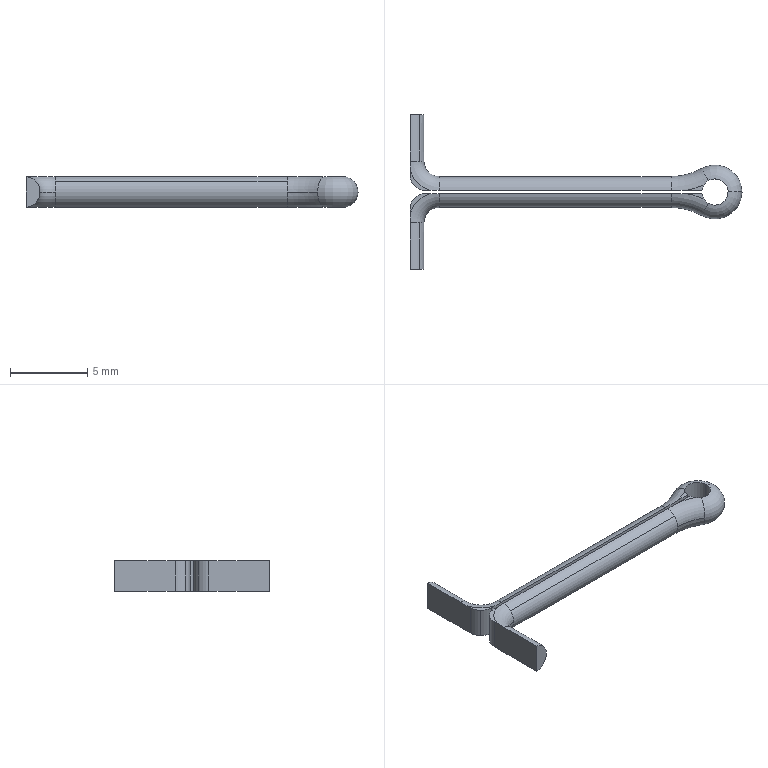Part | SolidWorks | features BaseBody 1 | 1 solid | 38 faces | box 21.489 x 10 x 2 mm | volume 72.863 mm3 | cylinder 14 | plane 14 | torus 10 | commonest cylinder face diameters 2 x12 1.7 x2
STEP:
#1=CARTESIAN_POINT('',(-17.839,-0.1,0.005013));
#2=VERTEX_POINT('',#1);
#3=CARTESIAN_POINT('',(-17.839,-1.,1.));
#4=VERTEX_POINT('',#3);
#5=CARTESIAN_POINT('',(-17.839,0.,1.));
#6=DIRECTION('',(-1.,0.,0.));
#7=DIRECTION('',(0.,0.,-1.));
#8=AXIS2_PLACEMENT_3D('',#5,#6,#7);
#9=CIRCLE('',#8,1.);
#10=EDGE_CURVE('',#2,#4,#9,.T.);
#11=ORIENTED_EDGE('',*,*,#10,.T.);
#12=CARTESIAN_POINT('',(-18.839,-2.,1.));
#13=VERTEX_POINT('',#12);
#14=CARTESIAN_POINT('',(-17.839,-2.,1.));
#15=DIRECTION('',(0.,0.,1.));
#16=DIRECTION('',(1.,0.,0.));
#17=AXIS2_PLACEMENT_3D('',#14,#15,#16);
#18=CIRCLE('',#17,1.);
#19=EDGE_CURVE('',#4,#13,#18,.T.);
#20=ORIENTED_EDGE('',*,*,#19,.T.);
#21=CARTESIAN_POINT('',(-19.739,-2.,0.005013));
#22=VERTEX_POINT('',#21);
#23=CARTESIAN_POINT('',(-19.839,-2.,1.));
#24=DIRECTION('',(0.,1.,0.));
#25=DIRECTION('',(1.,0.,0.));
#26=AXIS2_PLACEMENT_3D('',#23,#24,#25);
#27=CIRCLE('',#26,1.);
#28=EDGE_CURVE('',#13,#22,#27,.T.);
#29=ORIENTED_EDGE('',*,*,#28,.T.);
#30=CARTESIAN_POINT('',(-19.739,-1.376,0.));
#31=VERTEX_POINT('',#30);
#32=CARTESIAN_POINT('',(-19.739,-2.,0.005013));
#33=CARTESIAN_POINT('',(-19.739,-1.792,0.005013));
#34=CARTESIAN_POINT('',(-19.739,-1.584,0.));
#35=CARTESIAN_POINT('',(-19.739,-1.376,0.));
#36=B_SPLINE_CURVE_WITH_KNOTS('',3,(#32,#33,#34,#35),.UNSPECIFIED.,.F.,.F.,(4,4),(0.,0.0006245),.UNSPECIFIED.);
#37=EDGE_CURVE('',#22,#31,#36,.T.);
#38=ORIENTED_EDGE('',*,*,#37,.T.);
#39=CARTESIAN_POINT('',(-18.464,-0.1,0.));
#40=VERTEX_POINT('',#39);
#41=CARTESIAN_POINT('',(-17.839,-2.,0.));
#42=DIRECTION('',(0.,0.,-1.));
#43=DIRECTION('',(-0.7071,0.7071,0.));
#44=AXIS2_PLACEMENT_3D('',#41,#42,#43);
#45=CIRCLE('',#44,2.);
#46=EDGE_CURVE('',#31,#40,#45,.T.);
#47=ORIENTED_EDGE('',*,*,#46,.T.);
#48=CARTESIAN_POINT('',(-18.464,-0.1,0.));
#49=CARTESIAN_POINT('',(-18.256,-0.1,0.));
#50=CARTESIAN_POINT('',(-18.048,-0.1,0.005013));
#51=CARTESIAN_POINT('',(-17.839,-0.1,0.005013));
#52=B_SPLINE_CURVE_WITH_KNOTS('',3,(#48,#49,#50,#51),.UNSPECIFIED.,.F.,.F.,(4,4),(0.,0.0006245),.UNSPECIFIED.);
#53=EDGE_CURVE('',#40,#2,#52,.T.);
#54=ORIENTED_EDGE('',*,*,#53,.T.);
#55=EDGE_LOOP('',(#11,#20,#29,#38,#47,#54));
#56=FACE_OUTER_BOUND('',#55,.T.);
#57=CARTESIAN_POINT('',(-17.839,-2.,1.));
#58=DIRECTION('',(0.,0.,1.));
#59=DIRECTION('',(1.,0.,0.));
#60=AXIS2_PLACEMENT_3D('',#57,#58,#59);
#61=TOROIDAL_SURFACE('',#60,2.,1.);
#62=ADVANCED_FACE('',(#56),#61,.T.);
#63=CARTESIAN_POINT('',(-2.839,-0.7071,1.707));
#64=VERTEX_POINT('',#63);
#65=CARTESIAN_POINT('',(-2.839,-1.,1.));
#66=VERTEX_POINT('',#65);
#67=CARTESIAN_POINT('',(-2.839,0.,1.));
#68=DIRECTION('',(1.,0.,0.));
#69=DIRECTION('',(0.,-1.,0.));
#70=AXIS2_PLACEMENT_3D('',#67,#68,#69);
#71=CIRCLE('',#70,1.);
#72=EDGE_CURVE('',#64,#66,#71,.T.);
#73=ORIENTED_EDGE('',*,*,#72,.T.);
#74=CARTESIAN_POINT('',(-0.8642,-1.522,1.));
#75=VERTEX_POINT('',#74);
#76=CARTESIAN_POINT('',(-2.839,-5.,1.));
#77=DIRECTION('',(0.,0.,-1.));
#78=DIRECTION('',(-1.,0.,0.));
#79=AXIS2_PLACEMENT_3D('',#76,#77,#78);
#80=CIRCLE('',#79,4.);
#81=EDGE_CURVE('',#66,#75,#80,.T.);
#82=ORIENTED_EDGE('',*,*,#81,.T.);
#83=CARTESIAN_POINT('',(-0.4197,-0.7391,1.995));
#84=VERTEX_POINT('',#83);
#85=CARTESIAN_POINT('',(-0.3704,-0.6522,1.));
#86=DIRECTION('',(-0.8696,0.4938,0.));
#87=DIRECTION('',(0.,0.,-1.));
#88=AXIS2_PLACEMENT_3D('',#85,#86,#87);
#89=CIRCLE('',#88,1.);
#90=EDGE_CURVE('',#75,#84,#89,.T.);
#91=ORIENTED_EDGE('',*,*,#90,.T.);
#92=CARTESIAN_POINT('',(-0.7014,-0.4802,2.));
#93=VERTEX_POINT('',#92);
#94=CARTESIAN_POINT('',(-0.4197,-0.7391,1.995));
#95=CARTESIAN_POINT('',(-0.5324,-0.6751,1.995));
#96=CARTESIAN_POINT('',(-0.6281,-0.5871,2.));
#97=CARTESIAN_POINT('',(-0.7014,-0.4802,2.));
#98=B_SPLINE_CURVE_WITH_KNOTS('',3,(#94,#95,#96,#97),.UNSPECIFIED.,.F.,.F.,(4,4),(0.,0.0003832),.UNSPECIFIED.);
#99=EDGE_CURVE('',#84,#93,#98,.T.);
#100=ORIENTED_EDGE('',*,*,#99,.T.);
#101=CARTESIAN_POINT('',(-1.844,-0.1,2.));
#102=VERTEX_POINT('',#101);
#103=CARTESIAN_POINT('',(-2.839,-5.,2.));
#104=DIRECTION('',(0.,0.,1.));
#105=DIRECTION('',(0.2554,0.9668,0.));
#106=AXIS2_PLACEMENT_3D('',#103,#104,#105);
#107=CIRCLE('',#106,5.);
#108=EDGE_CURVE('',#93,#102,#107,.T.);
#109=ORIENTED_EDGE('',*,*,#108,.T.);
#110=CARTESIAN_POINT('',(-2.839,-0.1,1.995));
#111=VERTEX_POINT('',#110);
#112=CARTESIAN_POINT('',(-1.844,-0.1,2.));
#113=CARTESIAN_POINT('',(-2.176,-0.1,2.));
#114=CARTESIAN_POINT('',(-2.508,-0.1,1.995));
#115=CARTESIAN_POINT('',(-2.839,-0.1,1.995));
#116=B_SPLINE_CURVE_WITH_KNOTS('',3,(#112,#113,#114,#115),.UNSPECIFIED.,.F.,.F.,(4,4),(0.,0.000995),.UNSPECIFIED.);
#117=EDGE_CURVE('',#102,#111,#116,.T.);
#118=ORIENTED_EDGE('',*,*,#117,.T.);
#119=CARTESIAN_POINT('',(-2.839,0.,1.));
#120=DIRECTION('',(1.,0.,0.));
#121=DIRECTION('',(0.,-1.,0.));
#122=AXIS2_PLACEMENT_3D('',#119,#120,#121);
#123=CIRCLE('',#122,1.);
#124=EDGE_CURVE('',#111,#64,#123,.T.);
#125=ORIENTED_EDGE('',*,*,#124,.T.);
#126=EDGE_LOOP('',(#73,#82,#91,#100,#109,#118,#125));
#127=FACE_OUTER_BOUND('',#126,.T.);
#128=CARTESIAN_POINT('',(-2.839,-5.,1.));
#129=DIRECTION('',(0.,0.,-1.));
#130=DIRECTION('',(-1.,0.,0.));
#131=AXIS2_PLACEMENT_3D('',#128,#129,#130);
#132=TOROIDAL_SURFACE('',#131,5.,1.);
#133=ADVANCED_FACE('',(#127),#132,.T.);
#134=CARTESIAN_POINT('',(-0.4197,0.7391,1.995));
#135=VERTEX_POINT('',#134);
#136=CARTESIAN_POINT('',(-0.8642,1.522,1.));
#137=VERTEX_POINT('',#136);
#138=CARTESIAN_POINT('',(-0.3704,0.6522,1.));
#139=DIRECTION('',(-0.8696,-0.4938,0.));
#140=DIRECTION('',(-0.4938,0.8696,0.));
#141=AXIS2_PLACEMENT_3D('',#138,#139,#140);
#142=CIRCLE('',#141,1.);
#143=EDGE_CURVE('',#135,#137,#142,.T.);
#144=ORIENTED_EDGE('',*,*,#143,.T.);
#145=CARTESIAN_POINT('',(-2.839,1.,1.));
#146=VERTEX_POINT('',#145);
#147=CARTESIAN_POINT('',(-2.839,5.,1.));
#148=DIRECTION('',(0.,0.,-1.));
#149=DIRECTION('',(-1.,0.,0.));
#150=AXIS2_PLACEMENT_3D('',#147,#148,#149);
#151=CIRCLE('',#150,4.);
#152=EDGE_CURVE('',#137,#146,#151,.T.);
#153=ORIENTED_EDGE('',*,*,#152,.T.);
#154=CARTESIAN_POINT('',(-2.839,0.7071,1.707));
#155=VERTEX_POINT('',#154);
#156=CARTESIAN_POINT('',(-2.839,0.,1.));
#157=DIRECTION('',(1.,0.,0.));
#158=DIRECTION('',(0.,0.,-1.));
#159=AXIS2_PLACEMENT_3D('',#156,#157,#158);
#160=CIRCLE('',#159,1.);
#161=EDGE_CURVE('',#146,#155,#160,.T.);
#162=ORIENTED_EDGE('',*,*,#161,.T.);
#163=CARTESIAN_POINT('',(-2.839,0.1,1.995));
#164=VERTEX_POINT('',#163);
#165=CARTESIAN_POINT('',(-2.839,0.,1.));
#166=DIRECTION('',(1.,0.,0.));
#167=DIRECTION('',(0.,0.,-1.));
#168=AXIS2_PLACEMENT_3D('',#165,#166,#167);
#169=CIRCLE('',#168,1.);
#170=EDGE_CURVE('',#155,#164,#169,.T.);
#171=ORIENTED_EDGE('',*,*,#170,.T.);
#172=CARTESIAN_POINT('',(-1.844,0.1,2.));
#173=VERTEX_POINT('',#172);
#174=CARTESIAN_POINT('',(-2.839,0.1,1.995));
#175=CARTESIAN_POINT('',(-2.508,0.1,1.995));
#176=CARTESIAN_POINT('',(-2.176,0.1,2.));
#177=CARTESIAN_POINT('',(-1.844,0.1,2.));
#178=B_SPLINE_CURVE_WITH_KNOTS('',3,(#174,#175,#176,#177),.UNSPECIFIED.,.F.,.F.,(4,4),(0.,0.000995),.UNSPECIFIED.);
#179=EDGE_CURVE('',#164,#173,#178,.T.);
#180=ORIENTED_EDGE('',*,*,#179,.T.);
#181=CARTESIAN_POINT('',(-0.7014,0.4802,2.));
#182=VERTEX_POINT('',#181);
#183=CARTESIAN_POINT('',(-2.839,5.,2.));
#184=DIRECTION('',(0.,0.,1.));
#185=DIRECTION('',(0.2554,-0.9668,0.));
#186=AXIS2_PLACEMENT_3D('',#183,#184,#185);
#187=CIRCLE('',#186,5.);
#188=EDGE_CURVE('',#173,#182,#187,.T.);
#189=ORIENTED_EDGE('',*,*,#188,.T.);
#190=CARTESIAN_POINT('',(-0.7014,0.4802,2.));
#191=CARTESIAN_POINT('',(-0.6281,0.5871,2.));
#192=CARTESIAN_POINT('',(-0.5324,0.6751,1.995));
#193=CARTESIAN_POINT('',(-0.4197,0.7391,1.995));
#194=B_SPLINE_CURVE_WITH_KNOTS('',3,(#190,#191,#192,#193),.UNSPECIFIED.,.F.,.F.,(4,4),(0.,0.0003832),.UNSPECIFIED.);
#195=EDGE_CURVE('',#182,#135,#194,.T.);
#196=ORIENTED_EDGE('',*,*,#195,.T.);
#197=EDGE_LOOP('',(#144,#153,#162,#171,#180,#189,#196));
#198=FACE_OUTER_BOUND('',#197,.T.);
#199=CARTESIAN_POINT('',(-2.839,5.,1.));
#200=DIRECTION('',(0.,0.,-1.));
#201=DIRECTION('',(-1.,0.,0.));
#202=AXIS2_PLACEMENT_3D('',#199,#200,#201);
#203=TOROIDAL_SURFACE('',#202,5.,1.);
#204=ADVANCED_FACE('',(#198),#203,.T.);
#205=CARTESIAN_POINT('',(-19.739,2.,0.005013));
#206=VERTEX_POINT('',#205);
#207=CARTESIAN_POINT('',(-18.839,2.,1.));
#208=VERTEX_POINT('',#207);
#209=CARTESIAN_POINT('',(-19.839,2.,1.));
#210=DIRECTION('',(0.,-1.,0.));
#211=DIRECTION('',(0.,0.,-1.));
#212=AXIS2_PLACEMENT_3D('',#209,#210,#211);
#213=CIRCLE('',#212,1.);
#214=EDGE_CURVE('',#206,#208,#213,.T.);
#215=ORIENTED_EDGE('',*,*,#214,.T.);
#216=CARTESIAN_POINT('',(-17.839,1.,1.));
#217=VERTEX_POINT('',#216);
#218=CARTESIAN_POINT('',(-17.839,2.,1.));
#219=DIRECTION('',(0.,0.,1.));
#220=DIRECTION('',(1.,0.,0.));
#221=AXIS2_PLACEMENT_3D('',#218,#219,#220);
#222=CIRCLE('',#221,1.);
#223=EDGE_CURVE('',#208,#217,#222,.T.);
#224=ORIENTED_EDGE('',*,*,#223,.T.);
#225=CARTESIAN_POINT('',(-17.839,0.1,0.005013));
#226=VERTEX_POINT('',#225);
#227=CARTESIAN_POINT('',(-17.839,0.,1.));
#228=DIRECTION('',(-1.,0.,0.));
#229=DIRECTION('',(0.,1.,0.));
#230=AXIS2_PLACEMENT_3D('',#227,#228,#229);
#231=CIRCLE('',#230,1.);
#232=EDGE_CURVE('',#217,#226,#231,.T.);
#233=ORIENTED_EDGE('',*,*,#232,.T.);
#234=CARTESIAN_POINT('',(-18.464,0.1,0.));
#235=VERTEX_POINT('',#234);
#236=CARTESIAN_POINT('',(-17.839,0.1,0.005013));
#237=CARTESIAN_POINT('',(-18.048,0.1,0.005013));
#238=CARTESIAN_POINT('',(-18.256,0.1,0.));
#239=CARTESIAN_POINT('',(-18.464,0.1,0.));
#240=B_SPLINE_CURVE_WITH_KNOTS('',3,(#236,#237,#238,#239),.UNSPECIFIED.,.F.,.F.,(4,4),(0.,0.0006245),.UNSPECIFIED.);
#241=EDGE_CURVE('',#226,#235,#240,.T.);
#242=ORIENTED_EDGE('',*,*,#241,.T.);
#243=CARTESIAN_POINT('',(-19.739,1.376,0.));
#244=VERTEX_POINT('',#243);
#245=CARTESIAN_POINT('',(-17.839,2.,0.));
#246=DIRECTION('',(0.,0.,-1.));
#247=DIRECTION('',(-0.7071,-0.7071,0.));
#248=AXIS2_PLACEMENT_3D('',#245,#246,#247);
#249=CIRCLE('',#248,2.);
#250=EDGE_CURVE('',#235,#244,#249,.T.);
#251=ORIENTED_EDGE('',*,*,#250,.T.);
#252=CARTESIAN_POINT('',(-19.739,1.376,0.));
#253=CARTESIAN_POINT('',(-19.739,1.584,0.));
#254=CARTESIAN_POINT('',(-19.739,1.792,0.005013));
#255=CARTESIAN_POINT('',(-19.739,2.,0.005013));
#256=B_SPLINE_CURVE_WITH_KNOTS('',3,(#252,#253,#254,#255),.UNSPECIFIED.,.F.,.F.,(4,4),(0.,0.0006245),.UNSPECIFIED.);
#257=EDGE_CURVE('',#244,#206,#256,.T.);
#258=ORIENTED_EDGE('',*,*,#257,.T.);
#259=EDGE_LOOP('',(#215,#224,#233,#242,#251,#258));
#260=FACE_OUTER_BOUND('',#259,.T.);
#261=CARTESIAN_POINT('',(-17.839,2.,1.));
#262=DIRECTION('',(0.,0.,1.));
#263=DIRECTION('',(1.,0.,0.));
#264=AXIS2_PLACEMENT_3D('',#261,#262,#263);
#265=TOROIDAL_SURFACE('',#264,2.,1.);
#266=ADVANCED_FACE('',(#260),#265,.T.);
#267=CARTESIAN_POINT('',(-19.132,-2.,1.707));
#268=VERTEX_POINT('',#267);
#269=CARTESIAN_POINT('',(-19.839,-2.,1.));
#270=DIRECTION('',(0.,1.,0.));
#271=DIRECTION('',(1.,0.,0.));
#272=AXIS2_PLACEMENT_3D('',#269,#270,#271);
#273=CIRCLE('',#272,1.);
#274=EDGE_CURVE('',#268,#13,#273,.T.);
#275=ORIENTED_EDGE('',*,*,#274,.F.);
#276=CARTESIAN_POINT('',(-19.132,-5.,1.707));
#277=VERTEX_POINT('',#276);
#278=CARTESIAN_POINT('',(-19.132,-3.062,1.707));
#279=DIRECTION('',(0.,-1.,0.));
#280=VECTOR('',#279,1000.);
#281=LINE('',#278,#280);
#282=EDGE_CURVE('',#268,#277,#281,.T.);
#283=ORIENTED_EDGE('',*,*,#282,.T.);
#284=CARTESIAN_POINT('',(-19.739,-5.,0.005013));
#285=VERTEX_POINT('',#284);
#286=CARTESIAN_POINT('',(-19.839,-5.,1.));
#287=DIRECTION('',(0.,1.,0.));
#288=DIRECTION('',(0.7071,0.,0.7071));
#289=AXIS2_PLACEMENT_3D('',#286,#287,#288);
#290=CIRCLE('',#289,1.);
#291=EDGE_CURVE('',#277,#285,#290,.T.);
#292=ORIENTED_EDGE('',*,*,#291,.T.);
#293=CARTESIAN_POINT('',(-19.739,-3.062,0.005013));
#294=DIRECTION('',(0.,1.,0.));
#295=VECTOR('',#294,1000.);
#296=LINE('',#293,#295);
#297=EDGE_CURVE('',#285,#22,#296,.T.);
#298=ORIENTED_EDGE('',*,*,#297,.T.);
#299=ORIENTED_EDGE('',*,*,#28,.F.);
#300=EDGE_LOOP('',(#275,#283,#292,#298,#299));
#301=FACE_OUTER_BOUND('',#300,.T.);
#302=CARTESIAN_POINT('',(-19.839,-3.062,1.));
#303=DIRECTION('',(0.,-1.,0.));
#304=DIRECTION('',(0.7071,0.,0.7071));
#305=AXIS2_PLACEMENT_3D('',#302,#303,#304);
#306=CYLINDRICAL_SURFACE('',#305,1.);
#307=ADVANCED_FACE('',(#301),#306,.T.);
#308=ORIENTED_EDGE('',*,*,#72,.F.);
#309=CARTESIAN_POINT('',(-17.839,-0.7071,1.707));
#310=VERTEX_POINT('',#309);
#311=CARTESIAN_POINT('',(-10.341,-0.7071,1.707));
#312=DIRECTION('',(-1.,0.,0.));
#313=VECTOR('',#312,1000.);
#314=LINE('',#311,#313);
#315=EDGE_CURVE('',#64,#310,#314,.T.);
#316=ORIENTED_EDGE('',*,*,#315,.T.);
#317=CARTESIAN_POINT('',(-17.839,0.,1.));
#318=DIRECTION('',(-1.,0.,0.));
#319=DIRECTION('',(0.,0.,-1.));
#320=AXIS2_PLACEMENT_3D('',#317,#318,#319);
#321=CIRCLE('',#320,1.);
#322=EDGE_CURVE('',#4,#310,#321,.T.);
#323=ORIENTED_EDGE('',*,*,#322,.F.);
#324=ORIENTED_EDGE('',*,*,#10,.F.);
#325=CARTESIAN_POINT('',(-2.839,-0.1,0.005013));
#326=VERTEX_POINT('',#325);
#327=CARTESIAN_POINT('',(-10.341,-0.1,0.005013));
#328=DIRECTION('',(1.,0.,0.));
#329=VECTOR('',#328,1000.);
#330=LINE('',#327,#329);
#331=EDGE_CURVE('',#2,#326,#330,.T.);
#332=ORIENTED_EDGE('',*,*,#331,.T.);
#333=CARTESIAN_POINT('',(-2.839,0.,1.));
#334=DIRECTION('',(1.,0.,0.));
#335=DIRECTION('',(0.,-1.,0.));
#336=AXIS2_PLACEMENT_3D('',#333,#334,#335);
#337=CIRCLE('',#336,1.);
#338=EDGE_CURVE('',#66,#326,#337,.T.);
#339=ORIENTED_EDGE('',*,*,#338,.F.);
#340=EDGE_LOOP('',(#308,#316,#323,#324,#332,#339));
#341=FACE_OUTER_BOUND('',#340,.T.);
#342=CARTESIAN_POINT('',(-10.341,0.,1.));
#343=DIRECTION('',(-1.,0.,0.));
#344=DIRECTION('',(0.,-0.7071,0.7071));
#345=AXIS2_PLACEMENT_3D('',#342,#343,#344);
#346=CYLINDRICAL_SURFACE('',#345,1.);
#347=ADVANCED_FACE('',(#341),#346,.T.);
#348=CARTESIAN_POINT('',(-0.4197,-0.7391,0.005013));
#349=VERTEX_POINT('',#348);
#350=CARTESIAN_POINT('',(0.85,0.,0.005013));
#351=VERTEX_POINT('',#350);
#352=CARTESIAN_POINT('',(0.,0.,0.005013));
#353=DIRECTION('',(0.,0.,1.));
#354=DIRECTION('',(0.9931,0.1176,0.));
#355=AXIS2_PLACEMENT_3D('',#352,#353,#354);
#356=CIRCLE('',#355,0.85);
#357=EDGE_CURVE('',#349,#351,#356,.T.);
#358=ORIENTED_EDGE('',*,*,#357,.T.);
#359=CARTESIAN_POINT('',(0.85,0.,1.995));
#360=VERTEX_POINT('',#359);
#361=CARTESIAN_POINT('',(0.75,0.,1.));
#362=DIRECTION('',(0.,-1.,0.));
#363=DIRECTION('',(0.,0.,-1.));
#364=AXIS2_PLACEMENT_3D('',#361,#362,#363);
#365=CIRCLE('',#364,1.);
#366=EDGE_CURVE('',#351,#360,#365,.T.);
#367=ORIENTED_EDGE('',*,*,#366,.T.);
#368=CARTESIAN_POINT('',(0.,0.,1.995));
#369=DIRECTION('',(0.,0.,-1.));
#370=DIRECTION('',(0.9931,0.1176,0.));
#371=AXIS2_PLACEMENT_3D('',#368,#369,#370);
#372=CIRCLE('',#371,0.85);
#373=EDGE_CURVE('',#360,#84,#372,.T.);
#374=ORIENTED_EDGE('',*,*,#373,.T.);
#375=ORIENTED_EDGE('',*,*,#90,.F.);
#376=CARTESIAN_POINT('',(-0.3704,-0.6522,1.));
#377=DIRECTION('',(-0.8696,0.4938,0.));
#378=DIRECTION('',(0.,0.,-1.));
#379=AXIS2_PLACEMENT_3D('',#376,#377,#378);
#380=CIRCLE('',#379,1.);
#381=EDGE_CURVE('',#349,#75,#380,.T.);
#382=ORIENTED_EDGE('',*,*,#381,.F.);
#383=EDGE_LOOP('',(#358,#367,#374,#375,#382));
#384=FACE_OUTER_BOUND('',#383,.T.);
#385=CARTESIAN_POINT('',(0.,0.,1.));
#386=DIRECTION('',(0.,0.,1.));
#387=DIRECTION('',(1.,0.,0.));
#388=AXIS2_PLACEMENT_3D('',#385,#386,#387);
#389=TOROIDAL_SURFACE('',#388,0.75,1.);
#390=ADVANCED_FACE('',(#384),#389,.T.);
#391=CARTESIAN_POINT('',(-17.839,0.7071,1.707));
#392=VERTEX_POINT('',#391);
#393=CARTESIAN_POINT('',(-17.839,0.,1.));
#394=DIRECTION('',(-1.,0.,0.));
#395=DIRECTION('',(0.,1.,0.));
#396=AXIS2_PLACEMENT_3D('',#393,#394,#395);
#397=CIRCLE('',#396,1.);
#398=EDGE_CURVE('',#392,#217,#397,.T.);
#399=ORIENTED_EDGE('',*,*,#398,.F.);
#400=CARTESIAN_POINT('',(-1.639,0.7071,1.707));
#401=DIRECTION('',(1.,0.,0.));
#402=VECTOR('',#401,1000.);
#403=LINE('',#400,#402);
#404=EDGE_CURVE('',#392,#155,#403,.T.);
#405=ORIENTED_EDGE('',*,*,#404,.T.);
#406=ORIENTED_EDGE('',*,*,#161,.F.);
#407=CARTESIAN_POINT('',(-2.839,0.1,0.005013));
#408=VERTEX_POINT('',#407);
#409=CARTESIAN_POINT('',(-2.839,0.,1.));
#410=DIRECTION('',(1.,0.,0.));
#411=DIRECTION('',(0.,0.,-1.));
#412=AXIS2_PLACEMENT_3D('',#409,#410,#411);
#413=CIRCLE('',#412,1.);
#414=EDGE_CURVE('',#408,#146,#413,.T.);
#415=ORIENTED_EDGE('',*,*,#414,.F.);
#416=CARTESIAN_POINT('',(-1.639,0.1,0.005013));
#417=DIRECTION('',(-1.,0.,0.));
#418=VECTOR('',#417,1000.);
#419=LINE('',#416,#418);
#420=EDGE_CURVE('',#408,#226,#419,.T.);
#421=ORIENTED_EDGE('',*,*,#420,.T.);
#422=ORIENTED_EDGE('',*,*,#232,.F.);
#423=EDGE_LOOP('',(#399,#405,#406,#415,#421,#422));
#424=FACE_OUTER_BOUND('',#423,.T.);
#425=CARTESIAN_POINT('',(-1.639,0.,1.));
#426=DIRECTION('',(1.,0.,0.));
#427=DIRECTION('',(0.,0.7071,0.7071));
#428=AXIS2_PLACEMENT_3D('',#425,#426,#427);
#429=CYLINDRICAL_SURFACE('',#428,1.);
#430=ADVANCED_FACE('',(#424),#429,.T.);
#431=CARTESIAN_POINT('',(-19.739,5.,0.005013));
#432=VERTEX_POINT('',#431);
#433=CARTESIAN_POINT('',(-19.132,5.,1.707));
#434=VERTEX_POINT('',#433);
#435=CARTESIAN_POINT('',(-19.839,5.,1.));
#436=DIRECTION('',(0.,-1.,0.));
#437=DIRECTION('',(0.7071,0.,0.7071));
#438=AXIS2_PLACEMENT_3D('',#435,#436,#437);
#439=CIRCLE('',#438,1.);
#440=EDGE_CURVE('',#432,#434,#439,.T.);
#441=ORIENTED_EDGE('',*,*,#440,.T.);
#442=CARTESIAN_POINT('',(-19.132,2.,1.707));
#443=VERTEX_POINT('',#442);
#444=CARTESIAN_POINT('',(-19.132,-0.06177,1.707));
#445=DIRECTION('',(0.,-1.,0.));
#446=VECTOR('',#445,1000.);
#447=LINE('',#444,#446);
#448=EDGE_CURVE('',#434,#443,#447,.T.);
#449=ORIENTED_EDGE('',*,*,#448,.T.);
#450=CARTESIAN_POINT('',(-19.839,2.,1.));
#451=DIRECTION('',(0.,-1.,0.));
#452=DIRECTION('',(0.,0.,-1.));
#453=AXIS2_PLACEMENT_3D('',#450,#451,#452);
#454=CIRCLE('',#453,1.);
#455=EDGE_CURVE('',#208,#443,#454,.T.);
#456=ORIENTED_EDGE('',*,*,#455,.F.);
#457=ORIENTED_EDGE('',*,*,#214,.F.);
#458=CARTESIAN_POINT('',(-19.739,-0.06177,0.005013));
#459=DIRECTION('',(0.,1.,0.));
#460=VECTOR('',#459,1000.);
#461=LINE('',#458,#460);
#462=EDGE_CURVE('',#206,#432,#461,.T.);
#463=ORIENTED_EDGE('',*,*,#462,.T.);
#464=EDGE_LOOP('',(#441,#449,#456,#457,#463));
#465=FACE_OUTER_BOUND('',#464,.T.);
#466=CARTESIAN_POINT('',(-19.839,-0.06177,1.));
#467=DIRECTION('',(0.,-1.,0.));
#468=DIRECTION('',(0.7071,0.,0.7071));
#469=AXIS2_PLACEMENT_3D('',#466,#467,#468);
#470=CYLINDRICAL_SURFACE('',#469,1.);
#471=ADVANCED_FACE('',(#465),#470,.T.);
#472=CARTESIAN_POINT('',(0.8441,0.1,1.995));
#473=VERTEX_POINT('',#472);
#474=CARTESIAN_POINT('',(0.,0.,1.995));
#475=DIRECTION('',(0.,0.,-1.));
#476=DIRECTION('',(0.9931,0.1176,0.));
#477=AXIS2_PLACEMENT_3D('',#474,#475,#476);
#478=CIRCLE('',#477,0.85);
#479=EDGE_CURVE('',#473,#360,#478,.T.);
#480=ORIENTED_EDGE('',*,*,#479,.F.);
#481=CARTESIAN_POINT('',(0.8441,0.1,0.005013));
#482=VERTEX_POINT('',#481);
#483=CARTESIAN_POINT('',(0.8441,0.1,0.));
#484=DIRECTION('',(0.,0.,-1.));
#485=VECTOR('',#484,1000.);
#486=LINE('',#483,#485);
#487=EDGE_CURVE('',#473,#482,#486,.T.);
#488=ORIENTED_EDGE('',*,*,#487,.T.);
#489=CARTESIAN_POINT('',(0.,0.,0.005013));
#490=DIRECTION('',(0.,0.,1.));
#491=DIRECTION('',(0.9931,0.1176,0.));
#492=AXIS2_PLACEMENT_3D('',#489,#490,#491);
#493=CIRCLE('',#492,0.85);
#494=EDGE_CURVE('',#351,#482,#493,.T.);
#495=ORIENTED_EDGE('',*,*,#494,.F.);
#496=ORIENTED_EDGE('',*,*,#357,.F.);
#497=CARTESIAN_POINT('',(-0.7014,-0.4802,0.));
#498=VERTEX_POINT('',#497);
#499=CARTESIAN_POINT('',(-0.7014,-0.4802,0.));
#500=CARTESIAN_POINT('',(-0.6281,-0.5871,0.));
#501=CARTESIAN_POINT('',(-0.5324,-0.6751,0.005013));
#502=CARTESIAN_POINT('',(-0.4197,-0.7391,0.005013));
#503=B_SPLINE_CURVE_WITH_KNOTS('',3,(#499,#500,#501,#502),.UNSPECIFIED.,.F.,.F.,(4,4),(0.,0.0003832),.UNSPECIFIED.);
#504=EDGE_CURVE('',#498,#349,#503,.T.);
#505=ORIENTED_EDGE('',*,*,#504,.F.);
#506=CARTESIAN_POINT('',(-0.8441,-0.1,0.));
#507=VERTEX_POINT('',#506);
#508=CARTESIAN_POINT('',(0.,0.,0.));
#509=DIRECTION('',(0.,0.,-1.));
#510=DIRECTION('',(0.9931,0.1176,0.));
#511=AXIS2_PLACEMENT_3D('',#508,#509,#510);
#512=CIRCLE('',#511,0.85);
#513=EDGE_CURVE('',#498,#507,#512,.T.);
#514=ORIENTED_EDGE('',*,*,#513,.T.);
#515=CARTESIAN_POINT('',(-0.8441,-0.1,2.));
#516=VERTEX_POINT('',#515);
#517=CARTESIAN_POINT('',(-0.8441,-0.1,0.));
#518=DIRECTION('',(0.,0.,1.));
#519=VECTOR('',#518,1000.);
#520=LINE('',#517,#519);
#521=EDGE_CURVE('',#507,#516,#520,.T.);
#522=ORIENTED_EDGE('',*,*,#521,.T.);
#523=CARTESIAN_POINT('',(0.,0.,2.));
#524=DIRECTION('',(0.,0.,-1.));
#525=DIRECTION('',(0.9931,0.1176,0.));
#526=AXIS2_PLACEMENT_3D('',#523,#524,#525);
#527=CIRCLE('',#526,0.85);
#528=EDGE_CURVE('',#93,#516,#527,.T.);
#529=ORIENTED_EDGE('',*,*,#528,.F.);
#530=ORIENTED_EDGE('',*,*,#99,.F.);
#531=ORIENTED_EDGE('',*,*,#373,.F.);
#532=EDGE_LOOP('',(#480,#488,#495,#496,#505,#514,#522,#529,#530,#531));
#533=FACE_OUTER_BOUND('',#532,.T.);
#534=CARTESIAN_POINT('',(0.,0.,0.));
#535=DIRECTION('',(0.,0.,-1.));
#536=DIRECTION('',(0.9931,0.1176,0.));
#537=AXIS2_PLACEMENT_3D('',#534,#535,#536);
#538=CYLINDRICAL_SURFACE('',#537,0.85);
#539=ADVANCED_FACE('',(#533),#538,.F.);
#540=CARTESIAN_POINT('',(-19.739,-1.1,2.));
#541=VERTEX_POINT('',#540);
#542=CARTESIAN_POINT('',(-19.447,-0.3929,2.));
#543=VERTEX_POINT('',#542);
#544=CARTESIAN_POINT('',(-18.739,-1.1,2.));
#545=DIRECTION('',(0.,0.,-1.));
#546=DIRECTION('',(-0.7071,0.7071,0.));
#547=AXIS2_PLACEMENT_3D('',#544,#545,#546);
#548=CIRCLE('',#547,1.);
#549=EDGE_CURVE('',#541,#543,#548,.T.);
#550=ORIENTED_EDGE('',*,*,#549,.T.);
#551=CARTESIAN_POINT('',(-19.447,-0.3929,0.));
#552=VERTEX_POINT('',#551);
#553=CARTESIAN_POINT('',(-19.447,-0.3929,0.));
#554=DIRECTION('',(0.,0.,-1.));
#555=VECTOR('',#554,1000.);
#556=LINE('',#553,#555);
#557=EDGE_CURVE('',#543,#552,#556,.T.);
#558=ORIENTED_EDGE('',*,*,#557,.T.);
#559=CARTESIAN_POINT('',(-19.739,-1.1,0.));
#560=VERTEX_POINT('',#559);
#561=CARTESIAN_POINT('',(-18.739,-1.1,0.));
#562=DIRECTION('',(0.,0.,1.));
#563=DIRECTION('',(-0.7071,0.7071,0.));
#564=AXIS2_PLACEMENT_3D('',#561,#562,#563);
#565=CIRCLE('',#564,1.);
#566=EDGE_CURVE('',#552,#560,#565,.T.);
#567=ORIENTED_EDGE('',*,*,#566,.T.);
#568=CARTESIAN_POINT('',(-19.739,-1.1,0.));
#569=DIRECTION('',(0.,0.,1.));
#570=VECTOR('',#569,1000.);
#571=LINE('',#568,#570);
#572=EDGE_CURVE('',#560,#541,#571,.T.);
#573=ORIENTED_EDGE('',*,*,#572,.T.);
#574=EDGE_LOOP('',(#550,#558,#567,#573));
#575=FACE_OUTER_BOUND('',#574,.T.);
#576=CARTESIAN_POINT('',(-18.739,-1.1,0.));
#577=DIRECTION('',(0.,0.,-1.));
#578=DIRECTION('',(-0.7071,0.7071,0.));
#579=AXIS2_PLACEMENT_3D('',#576,#577,#578);
#580=CYLINDRICAL_SURFACE('',#579,1.);
#581=ADVANCED_FACE('',(#575),#580,.T.);
#582=CARTESIAN_POINT('',(-18.739,0.1,2.));
#583=VERTEX_POINT('',#582);
#584=CARTESIAN_POINT('',(-19.447,0.3929,2.));
#585=VERTEX_POINT('',#584);
#586=CARTESIAN_POINT('',(-18.739,1.1,2.));
#587=DIRECTION('',(0.,0.,-1.));
#588=DIRECTION('',(-0.7071,-0.7071,0.));
#589=AXIS2_PLACEMENT_3D('',#586,#587,#588);
#590=CIRCLE('',#589,1.);
#591=EDGE_CURVE('',#583,#585,#590,.T.);
#592=ORIENTED_EDGE('',*,*,#591,.T.);
#593=CARTESIAN_POINT('',(-19.447,0.3929,0.));
#594=VERTEX_POINT('',#593);
#595=CARTESIAN_POINT('',(-19.447,0.3929,0.));
#596=DIRECTION('',(0.,0.,-1.));
#597=VECTOR('',#596,1000.);
#598=LINE('',#595,#597);
#599=EDGE_CURVE('',#585,#594,#598,.T.);
#600=ORIENTED_EDGE('',*,*,#599,.T.);
#601=CARTESIAN_POINT('',(-18.739,0.1,0.));
#602=VERTEX_POINT('',#601);
#603=CARTESIAN_POINT('',(-18.739,1.1,0.));
#604=DIRECTION('',(0.,0.,1.));
#605=DIRECTION('',(-0.7071,-0.7071,0.));
#606=AXIS2_PLACEMENT_3D('',#603,#604,#605);
#607=CIRCLE('',#606,1.);
#608=EDGE_CURVE('',#594,#602,#607,.T.);
#609=ORIENTED_EDGE('',*,*,#608,.T.);
#610=CARTESIAN_POINT('',(-18.739,0.1,0.));
#611=DIRECTION('',(0.,0.,1.));
#612=VECTOR('',#611,1000.);
#613=LINE('',#610,#612);
#614=EDGE_CURVE('',#602,#583,#613,.T.);
#615=ORIENTED_EDGE('',*,*,#614,.T.);
#616=EDGE_LOOP('',(#592,#600,#609,#615));
#617=FACE_OUTER_BOUND('',#616,.T.);
#618=CARTESIAN_POINT('',(-18.739,1.1,0.));
#619=DIRECTION('',(0.,0.,-1.));
#620=DIRECTION('',(-0.7071,-0.7071,0.));
#621=AXIS2_PLACEMENT_3D('',#618,#619,#620);
#622=CYLINDRICAL_SURFACE('',#621,1.);
#623=ADVANCED_FACE('',(#617),#622,.T.);
#624=ORIENTED_EDGE('',*,*,#37,.F.);
#625=ORIENTED_EDGE('',*,*,#297,.F.);
#626=CARTESIAN_POINT('',(-19.739,-5.,1.995));
#627=VERTEX_POINT('',#626);
#628=CARTESIAN_POINT('',(-19.739,-5.,0.));
#629=DIRECTION('',(0.,0.,1.));
#630=VECTOR('',#629,1000.);
#631=LINE('',#628,#630);
#632=EDGE_CURVE('',#285,#627,#631,.T.);
#633=ORIENTED_EDGE('',*,*,#632,.T.);
#634=CARTESIAN_POINT('',(-19.739,-2.,1.995));
#635=VERTEX_POINT('',#634);
#636=CARTESIAN_POINT('',(-19.739,-3.062,1.995));
#637=DIRECTION('',(0.,-1.,0.));
#638=VECTOR('',#637,1000.);
#639=LINE('',#636,#638);
#640=EDGE_CURVE('',#635,#627,#639,.T.);
#641=ORIENTED_EDGE('',*,*,#640,.F.);
#642=CARTESIAN_POINT('',(-19.739,-1.376,2.));
#643=VERTEX_POINT('',#642);
#644=CARTESIAN_POINT('',(-19.739,-1.376,2.));
#645=CARTESIAN_POINT('',(-19.739,-1.584,2.));
#646=CARTESIAN_POINT('',(-19.739,-1.792,1.995));
#647=CARTESIAN_POINT('',(-19.739,-2.,1.995));
#648=B_SPLINE_CURVE_WITH_KNOTS('',3,(#644,#645,#646,#647),.UNSPECIFIED.,.F.,.F.,(4,4),(0.,0.0006245),.UNSPECIFIED.);
#649=EDGE_CURVE('',#643,#635,#648,.T.);
#650=ORIENTED_EDGE('',*,*,#649,.F.);
#651=CARTESIAN_POINT('',(-19.739,-0.1,2.));
#652=DIRECTION('',(0.,-1.,0.));
#653=VECTOR('',#652,1000.);
#654=LINE('',#651,#653);
#655=EDGE_CURVE('',#541,#643,#654,.T.);
#656=ORIENTED_EDGE('',*,*,#655,.F.);
#657=ORIENTED_EDGE('',*,*,#572,.F.);
#658=CARTESIAN_POINT('',(-19.739,-0.1,0.));
#659=DIRECTION('',(0.,-1.,0.));
#660=VECTOR('',#659,1000.);
#661=LINE('',#658,#660);
#662=EDGE_CURVE('',#560,#31,#661,.T.);
#663=ORIENTED_EDGE('',*,*,#662,.T.);
#664=EDGE_LOOP('',(#624,#625,#633,#641,#650,#656,#657,#663));
#665=FACE_OUTER_BOUND('',#664,.T.);
#666=CARTESIAN_POINT('',(-19.739,-0.1,0.));
#667=DIRECTION('',(-1.,0.,0.));
#668=DIRECTION('',(0.,0.,1.));
#669=AXIS2_PLACEMENT_3D('',#666,#667,#668);
#670=PLANE('',#669);
#671=ADVANCED_FACE('',(#665),#670,.T.);
#672=CARTESIAN_POINT('',(-19.839,-5.,1.));
#673=DIRECTION('',(0.,1.,0.));
#674=DIRECTION('',(0.7071,0.,0.7071));
#675=AXIS2_PLACEMENT_3D('',#672,#673,#674);
#676=CIRCLE('',#675,1.);
#677=EDGE_CURVE('',#627,#277,#676,.T.);
#678=ORIENTED_EDGE('',*,*,#677,.F.);
#679=ORIENTED_EDGE('',*,*,#632,.F.);
#680=ORIENTED_EDGE('',*,*,#291,.F.);
#681=EDGE_LOOP('',(#678,#679,#680));
#682=FACE_OUTER_BOUND('',#681,.T.);
#683=CARTESIAN_POINT('',(-19.739,-5.,0.));
#684=DIRECTION('',(0.,-1.,0.));
#685=DIRECTION('',(-1.,0.,0.));
#686=AXIS2_PLACEMENT_3D('',#683,#684,#685);
#687=PLANE('',#686);
#688=ADVANCED_FACE('',(#682),#687,.T.);
#689=ORIENTED_EDGE('',*,*,#250,.F.);
#690=CARTESIAN_POINT('',(-19.739,0.1,0.));
#691=DIRECTION('',(1.,0.,0.));
#692=VECTOR('',#691,1000.);
#693=LINE('',#690,#692);
#694=EDGE_CURVE('',#602,#235,#693,.T.);
#695=ORIENTED_EDGE('',*,*,#694,.F.);
#696=ORIENTED_EDGE('',*,*,#608,.F.);
#697=CARTESIAN_POINT('',(-19.739,1.1,0.));
#698=VERTEX_POINT('',#697);
#699=CARTESIAN_POINT('',(-18.739,1.1,0.));
#700=DIRECTION('',(0.,0.,1.));
#701=DIRECTION('',(-0.7071,-0.7071,0.));
#702=AXIS2_PLACEMENT_3D('',#699,#700,#701);
#703=CIRCLE('',#702,1.);
#704=EDGE_CURVE('',#698,#594,#703,.T.);
#705=ORIENTED_EDGE('',*,*,#704,.F.);
#706=CARTESIAN_POINT('',(-19.739,5.,0.));
#707=DIRECTION('',(0.,-1.,0.));
#708=VECTOR('',#707,1000.);
#709=LINE('',#706,#708);
#710=EDGE_CURVE('',#244,#698,#709,.T.);
#711=ORIENTED_EDGE('',*,*,#710,.F.);
#712=EDGE_LOOP('',(#689,#695,#696,#705,#711));
#713=FACE_OUTER_BOUND('',#712,.T.);
#714=CARTESIAN_POINT('',(-1.842,-1.124,0.));
#715=DIRECTION('',(0.,0.,1.));
#716=DIRECTION('',(1.,0.,0.));
#717=AXIS2_PLACEMENT_3D('',#714,#715,#716);
#718=PLANE('',#717);
#719=ADVANCED_FACE('',(#713),#718,.F.);
#720=CARTESIAN_POINT('',(-0.7014,0.4802,0.));
#721=VERTEX_POINT('',#720);
#722=CARTESIAN_POINT('',(-1.844,0.1,0.));
#723=VERTEX_POINT('',#722);
#724=CARTESIAN_POINT('',(-2.839,5.,0.));
#725=DIRECTION('',(0.,0.,-1.));
#726=DIRECTION('',(0.2554,-0.9668,0.));
#727=AXIS2_PLACEMENT_3D('',#724,#725,#726);
#728=CIRCLE('',#727,5.);
#729=EDGE_CURVE('',#721,#723,#728,.T.);
#730=ORIENTED_EDGE('',*,*,#729,.F.);
#731=CARTESIAN_POINT('',(-0.8441,0.1,0.));
#732=VERTEX_POINT('',#731);
#733=CARTESIAN_POINT('',(0.,0.,0.));
#734=DIRECTION('',(0.,0.,-1.));
#735=DIRECTION('',(0.9931,0.1176,0.));
#736=AXIS2_PLACEMENT_3D('',#733,#734,#735);
#737=CIRCLE('',#736,0.85);
#738=EDGE_CURVE('',#732,#721,#737,.T.);
#739=ORIENTED_EDGE('',*,*,#738,.F.);
#740=CARTESIAN_POINT('',(-19.739,0.1,0.));
#741=DIRECTION('',(1.,0.,0.));
#742=VECTOR('',#741,1000.);
#743=LINE('',#740,#742);
#744=EDGE_CURVE('',#723,#732,#743,.T.);
#745=ORIENTED_EDGE('',*,*,#744,.F.);
#746=EDGE_LOOP('',(#730,#739,#745));
#747=FACE_OUTER_BOUND('',#746,.T.);
#748=CARTESIAN_POINT('',(-1.842,-1.124,0.));
#749=DIRECTION('',(0.,0.,1.));
#750=DIRECTION('',(1.,0.,0.));
#751=AXIS2_PLACEMENT_3D('',#748,#749,#750);
#752=PLANE('',#751);
#753=ADVANCED_FACE('',(#747),#752,.F.);
#754=CARTESIAN_POINT('',(-1.844,-0.1,0.));
#755=VERTEX_POINT('',#754);
#756=CARTESIAN_POINT('',(-2.839,-5.,0.));
#757=DIRECTION('',(0.,0.,-1.));
#758=DIRECTION('',(0.2554,0.9668,0.));
#759=AXIS2_PLACEMENT_3D('',#756,#757,#758);
#760=CIRCLE('',#759,5.);
#761=EDGE_CURVE('',#755,#498,#760,.T.);
#762=ORIENTED_EDGE('',*,*,#761,.F.);
#763=CARTESIAN_POINT('',(-0.8441,-0.1,0.));
#764=DIRECTION('',(-1.,0.,0.));
#765=VECTOR('',#764,1000.);
#766=LINE('',#763,#765);
#767=EDGE_CURVE('',#507,#755,#766,.T.);
#768=ORIENTED_EDGE('',*,*,#767,.F.);
#769=ORIENTED_EDGE('',*,*,#513,.F.);
#770=EDGE_LOOP('',(#762,#768,#769));
#771=FACE_OUTER_BOUND('',#770,.T.);
#772=CARTESIAN_POINT('',(-1.842,-1.124,0.));
#773=DIRECTION('',(0.,0.,1.));
#774=DIRECTION('',(1.,0.,0.));
#775=AXIS2_PLACEMENT_3D('',#772,#773,#774);
#776=PLANE('',#775);
#777=ADVANCED_FACE('',(#771),#776,.F.);
#778=ORIENTED_EDGE('',*,*,#53,.F.);
#779=CARTESIAN_POINT('',(-18.739,-0.1,0.));
#780=VERTEX_POINT('',#779);
#781=CARTESIAN_POINT('',(-0.8441,-0.1,0.));
#782=DIRECTION('',(-1.,0.,0.));
#783=VECTOR('',#782,1000.);
#784=LINE('',#781,#783);
#785=EDGE_CURVE('',#40,#780,#784,.T.);
#786=ORIENTED_EDGE('',*,*,#785,.T.);
#787=CARTESIAN_POINT('',(-18.739,-0.1,2.));
#788=VERTEX_POINT('',#787);
#789=CARTESIAN_POINT('',(-18.739,-0.1,0.));
#790=DIRECTION('',(0.,0.,-1.));
#791=VECTOR('',#790,1000.);
#792=LINE('',#789,#791);
#793=EDGE_CURVE('',#788,#780,#792,.T.);
#794=ORIENTED_EDGE('',*,*,#793,.F.);
#795=CARTESIAN_POINT('',(-18.464,-0.1,2.));
#796=VERTEX_POINT('',#795);
#797=CARTESIAN_POINT('',(-0.8441,-0.1,2.));
#798=DIRECTION('',(-1.,0.,0.));
#799=VECTOR('',#798,1000.);
#800=LINE('',#797,#799);
#801=EDGE_CURVE('',#796,#788,#800,.T.);
#802=ORIENTED_EDGE('',*,*,#801,.F.);
#803=CARTESIAN_POINT('',(-17.839,-0.1,1.995));
#804=VERTEX_POINT('',#803);
#805=CARTESIAN_POINT('',(-17.839,-0.1,1.995));
#806=CARTESIAN_POINT('',(-18.048,-0.1,1.995));
#807=CARTESIAN_POINT('',(-18.256,-0.1,2.));
#808=CARTESIAN_POINT('',(-18.464,-0.1,2.));
#809=B_SPLINE_CURVE_WITH_KNOTS('',3,(#805,#806,#807,#808),.UNSPECIFIED.,.F.,.F.,(4,4),(0.,0.0006245),.UNSPECIFIED.);
#810=EDGE_CURVE('',#804,#796,#809,.T.);
#811=ORIENTED_EDGE('',*,*,#810,.F.);
#812=CARTESIAN_POINT('',(-10.341,-0.1,1.995));
#813=DIRECTION('',(-1.,0.,0.));
#814=VECTOR('',#813,1000.);
#815=LINE('',#812,#814);
#816=EDGE_CURVE('',#111,#804,#815,.T.);
#817=ORIENTED_EDGE('',*,*,#816,.F.);
#818=ORIENTED_EDGE('',*,*,#117,.F.);
#819=CARTESIAN_POINT('',(-0.8441,-0.1,2.));
#820=DIRECTION('',(-1.,0.,0.));
#821=VECTOR('',#820,1000.);
#822=LINE('',#819,#821);
#823=EDGE_CURVE('',#516,#102,#822,.T.);
#824=ORIENTED_EDGE('',*,*,#823,.F.);
#825=ORIENTED_EDGE('',*,*,#521,.F.);
#826=ORIENTED_EDGE('',*,*,#767,.T.);
#827=CARTESIAN_POINT('',(-2.839,-0.1,0.005013));
#828=CARTESIAN_POINT('',(-2.508,-0.1,0.005013));
#829=CARTESIAN_POINT('',(-2.176,-0.1,0.));
#830=CARTESIAN_POINT('',(-1.844,-0.1,0.));
#831=B_SPLINE_CURVE_WITH_KNOTS('',3,(#827,#828,#829,#830),.UNSPECIFIED.,.F.,.F.,(4,4),(0.,0.000995),.UNSPECIFIED.);
#832=EDGE_CURVE('',#326,#755,#831,.T.);
#833=ORIENTED_EDGE('',*,*,#832,.F.);
#834=ORIENTED_EDGE('',*,*,#331,.F.);
#835=EDGE_LOOP('',(#778,#786,#794,#802,#811,#817,#818,#824,#825,#826,#833,#834));
#836=FACE_OUTER_BOUND('',#835,.T.);
#837=CARTESIAN_POINT('',(-0.8441,-0.1,0.));
#838=DIRECTION('',(0.,1.,0.));
#839=DIRECTION('',(1.,0.,0.));
#840=AXIS2_PLACEMENT_3D('',#837,#838,#839);
#841=PLANE('',#840);
#842=ADVANCED_FACE('',(#836),#841,.T.);
#843=CARTESIAN_POINT('',(-1.844,0.1,0.));
#844=CARTESIAN_POINT('',(-2.176,0.1,0.));
#845=CARTESIAN_POINT('',(-2.508,0.1,0.005013));
#846=CARTESIAN_POINT('',(-2.839,0.1,0.005013));
#847=B_SPLINE_CURVE_WITH_KNOTS('',3,(#843,#844,#845,#846),.UNSPECIFIED.,.F.,.F.,(4,4),(0.,0.000995),.UNSPECIFIED.);
#848=EDGE_CURVE('',#723,#408,#847,.T.);
#849=ORIENTED_EDGE('',*,*,#848,.F.);
#850=ORIENTED_EDGE('',*,*,#744,.T.);
#851=CARTESIAN_POINT('',(-0.8441,0.1,2.));
#852=VERTEX_POINT('',#851);
#853=CARTESIAN_POINT('',(-0.8441,0.1,0.));
#854=DIRECTION('',(0.,0.,1.));
#855=VECTOR('',#854,1000.);
#856=LINE('',#853,#855);
#857=EDGE_CURVE('',#732,#852,#856,.T.);
#858=ORIENTED_EDGE('',*,*,#857,.T.);
#859=CARTESIAN_POINT('',(-19.739,0.1,2.));
#860=DIRECTION('',(1.,0.,0.));
#861=VECTOR('',#860,1000.);
#862=LINE('',#859,#861);
#863=EDGE_CURVE('',#173,#852,#862,.T.);
#864=ORIENTED_EDGE('',*,*,#863,.F.);
#865=ORIENTED_EDGE('',*,*,#179,.F.);
#866=CARTESIAN_POINT('',(-17.839,0.1,1.995));
#867=VERTEX_POINT('',#866);
#868=CARTESIAN_POINT('',(-1.639,0.1,1.995));
#869=DIRECTION('',(1.,0.,0.));
#870=VECTOR('',#869,1000.);
#871=LINE('',#868,#870);
#872=EDGE_CURVE('',#867,#164,#871,.T.);
#873=ORIENTED_EDGE('',*,*,#872,.F.);
#874=CARTESIAN_POINT('',(-18.464,0.1,2.));
#875=VERTEX_POINT('',#874);
#876=CARTESIAN_POINT('',(-18.464,0.1,2.));
#877=CARTESIAN_POINT('',(-18.256,0.1,2.));
#878=CARTESIAN_POINT('',(-18.048,0.1,1.995));
#879=CARTESIAN_POINT('',(-17.839,0.1,1.995));
#880=B_SPLINE_CURVE_WITH_KNOTS('',3,(#876,#877,#878,#879),.UNSPECIFIED.,.F.,.F.,(4,4),(0.,0.0006245),.UNSPECIFIED.);
#881=EDGE_CURVE('',#875,#867,#880,.T.);
#882=ORIENTED_EDGE('',*,*,#881,.F.);
#883=CARTESIAN_POINT('',(-19.739,0.1,2.));
#884=DIRECTION('',(1.,0.,0.));
#885=VECTOR('',#884,1000.);
#886=LINE('',#883,#885);
#887=EDGE_CURVE('',#583,#875,#886,.T.);
#888=ORIENTED_EDGE('',*,*,#887,.F.);
#889=ORIENTED_EDGE('',*,*,#614,.F.);
#890=ORIENTED_EDGE('',*,*,#694,.T.);
#891=ORIENTED_EDGE('',*,*,#241,.F.);
#892=ORIENTED_EDGE('',*,*,#420,.F.);
#893=EDGE_LOOP('',(#849,#850,#858,#864,#865,#873,#882,#888,#889,#890,#891,#892));
#894=FACE_OUTER_BOUND('',#893,.T.);
#895=CARTESIAN_POINT('',(-19.739,0.1,0.));
#896=DIRECTION('',(0.,-1.,0.));
#897=DIRECTION('',(0.,0.,-1.));
#898=AXIS2_PLACEMENT_3D('',#895,#896,#897);
#899=PLANE('',#898);
#900=ADVANCED_FACE('',(#894),#899,.T.);
#901=ORIENTED_EDGE('',*,*,#108,.F.);
#902=ORIENTED_EDGE('',*,*,#528,.T.);
#903=ORIENTED_EDGE('',*,*,#823,.T.);
#904=EDGE_LOOP('',(#901,#902,#903));
#905=FACE_OUTER_BOUND('',#904,.T.);
#906=CARTESIAN_POINT('',(-1.842,-1.124,2.));
#907=DIRECTION('',(0.,0.,1.));
#908=DIRECTION('',(1.,0.,0.));
#909=AXIS2_PLACEMENT_3D('',#906,#907,#908);
#910=PLANE('',#909);
#911=ADVANCED_FACE('',(#905),#910,.T.);
#912=ORIENTED_EDGE('',*,*,#188,.F.);
#913=ORIENTED_EDGE('',*,*,#863,.T.);
#914=CARTESIAN_POINT('',(0.,0.,2.));
#915=DIRECTION('',(0.,0.,-1.));
#916=DIRECTION('',(0.9931,0.1176,0.));
#917=AXIS2_PLACEMENT_3D('',#914,#915,#916);
#918=CIRCLE('',#917,0.85);
#919=EDGE_CURVE('',#852,#182,#918,.T.);
#920=ORIENTED_EDGE('',*,*,#919,.T.);
#921=EDGE_LOOP('',(#912,#913,#920));
#922=FACE_OUTER_BOUND('',#921,.T.);
#923=CARTESIAN_POINT('',(-1.842,-1.124,2.));
#924=DIRECTION('',(0.,0.,1.));
#925=DIRECTION('',(1.,0.,0.));
#926=AXIS2_PLACEMENT_3D('',#923,#924,#925);
#927=PLANE('',#926);
#928=ADVANCED_FACE('',(#922),#927,.T.);
#929=CARTESIAN_POINT('',(-19.739,1.376,2.));
#930=VERTEX_POINT('',#929);
#931=CARTESIAN_POINT('',(-17.839,2.,2.));
#932=DIRECTION('',(0.,0.,1.));
#933=DIRECTION('',(-0.7071,-0.7071,0.));
#934=AXIS2_PLACEMENT_3D('',#931,#932,#933);
#935=CIRCLE('',#934,2.);
#936=EDGE_CURVE('',#930,#875,#935,.T.);
#937=ORIENTED_EDGE('',*,*,#936,.F.);
#938=CARTESIAN_POINT('',(-19.739,1.1,2.));
#939=VERTEX_POINT('',#938);
#940=CARTESIAN_POINT('',(-19.739,5.,2.));
#941=DIRECTION('',(0.,-1.,0.));
#942=VECTOR('',#941,1000.);
#943=LINE('',#940,#942);
#944=EDGE_CURVE('',#930,#939,#943,.T.);
#945=ORIENTED_EDGE('',*,*,#944,.T.);
#946=CARTESIAN_POINT('',(-18.739,1.1,2.));
#947=DIRECTION('',(0.,0.,-1.));
#948=DIRECTION('',(-0.7071,-0.7071,0.));
#949=AXIS2_PLACEMENT_3D('',#946,#947,#948);
#950=CIRCLE('',#949,1.);
#951=EDGE_CURVE('',#585,#939,#950,.T.);
#952=ORIENTED_EDGE('',*,*,#951,.F.);
#953=ORIENTED_EDGE('',*,*,#591,.F.);
#954=ORIENTED_EDGE('',*,*,#887,.T.);
#955=EDGE_LOOP('',(#937,#945,#952,#953,#954));
#956=FACE_OUTER_BOUND('',#955,.T.);
#957=CARTESIAN_POINT('',(-1.842,-1.124,2.));
#958=DIRECTION('',(0.,0.,1.));
#959=DIRECTION('',(1.,0.,0.));
#960=AXIS2_PLACEMENT_3D('',#957,#958,#959);
#961=PLANE('',#960);
#962=ADVANCED_FACE('',(#956),#961,.T.);
#963=CARTESIAN_POINT('',(-17.839,-2.,2.));
#964=DIRECTION('',(0.,0.,1.));
#965=DIRECTION('',(-0.7071,0.7071,0.));
#966=AXIS2_PLACEMENT_3D('',#963,#964,#965);
#967=CIRCLE('',#966,2.);
#968=EDGE_CURVE('',#796,#643,#967,.T.);
#969=ORIENTED_EDGE('',*,*,#968,.F.);
#970=ORIENTED_EDGE('',*,*,#801,.T.);
#971=CARTESIAN_POINT('',(-18.739,-1.1,2.));
#972=DIRECTION('',(0.,0.,-1.));
#973=DIRECTION('',(-0.7071,0.7071,0.));
#974=AXIS2_PLACEMENT_3D('',#971,#972,#973);
#975=CIRCLE('',#974,1.);
#976=EDGE_CURVE('',#543,#788,#975,.T.);
#977=ORIENTED_EDGE('',*,*,#976,.F.);
#978=ORIENTED_EDGE('',*,*,#549,.F.);
#979=ORIENTED_EDGE('',*,*,#655,.T.);
#980=EDGE_LOOP('',(#969,#970,#977,#978,#979));
#981=FACE_OUTER_BOUND('',#980,.T.);
#982=CARTESIAN_POINT('',(-1.842,-1.124,2.));
#983=DIRECTION('',(0.,0.,1.));
#984=DIRECTION('',(1.,0.,0.));
#985=AXIS2_PLACEMENT_3D('',#982,#983,#984);
#986=PLANE('',#985);
#987=ADVANCED_FACE('',(#981),#986,.T.);
#988=ORIENTED_EDGE('',*,*,#46,.F.);
#989=ORIENTED_EDGE('',*,*,#662,.F.);
#990=ORIENTED_EDGE('',*,*,#566,.F.);
#991=CARTESIAN_POINT('',(-18.739,-1.1,0.));
#992=DIRECTION('',(0.,0.,1.));
#993=DIRECTION('',(-0.7071,0.7071,0.));
#994=AXIS2_PLACEMENT_3D('',#991,#992,#993);
#995=CIRCLE('',#994,1.);
#996=EDGE_CURVE('',#780,#552,#995,.T.);
#997=ORIENTED_EDGE('',*,*,#996,.F.);
#998=ORIENTED_EDGE('',*,*,#785,.F.);
#999=EDGE_LOOP('',(#988,#989,#990,#997,#998));
#1000=FACE_OUTER_BOUND('',#999,.T.);
#1001=CARTESIAN_POINT('',(-1.842,-1.124,0.));
#1002=DIRECTION('',(0.,0.,1.));
#1003=DIRECTION('',(1.,0.,0.));
#1004=AXIS2_PLACEMENT_3D('',#1001,#1002,#1003);
#1005=PLANE('',#1004);
#1006=ADVANCED_FACE('',(#1000),#1005,.F.);
#1007=ORIENTED_EDGE('',*,*,#257,.F.);
#1008=ORIENTED_EDGE('',*,*,#710,.T.);
#1009=CARTESIAN_POINT('',(-19.739,1.1,0.));
#1010=DIRECTION('',(0.,0.,-1.));
#1011=VECTOR('',#1010,1000.);
#1012=LINE('',#1009,#1011);
#1013=EDGE_CURVE('',#939,#698,#1012,.T.);
#1014=ORIENTED_EDGE('',*,*,#1013,.F.);
#1015=ORIENTED_EDGE('',*,*,#944,.F.);
#1016=CARTESIAN_POINT('',(-19.739,2.,1.995));
#1017=VERTEX_POINT('',#1016);
#1018=CARTESIAN_POINT('',(-19.739,2.,1.995));
#1019=CARTESIAN_POINT('',(-19.739,1.792,1.995));
#1020=CARTESIAN_POINT('',(-19.739,1.584,2.));
#1021=CARTESIAN_POINT('',(-19.739,1.376,2.));
#1022=B_SPLINE_CURVE_WITH_KNOTS('',3,(#1018,#1019,#1020,#1021),.UNSPECIFIED.,.F.,.F.,(4,4),(0.,0.0006245),.UNSPECIFIED.);
#1023=EDGE_CURVE('',#1017,#930,#1022,.T.);
#1024=ORIENTED_EDGE('',*,*,#1023,.F.);
#1025=CARTESIAN_POINT('',(-19.739,5.,1.995));
#1026=VERTEX_POINT('',#1025);
#1027=CARTESIAN_POINT('',(-19.739,-0.06177,1.995));
#1028=DIRECTION('',(0.,-1.,0.));
#1029=VECTOR('',#1028,1000.);
#1030=LINE('',#1027,#1029);
#1031=EDGE_CURVE('',#1026,#1017,#1030,.T.);
#1032=ORIENTED_EDGE('',*,*,#1031,.F.);
#1033=CARTESIAN_POINT('',(-19.739,5.,0.));
#1034=DIRECTION('',(0.,0.,1.));
#1035=VECTOR('',#1034,1000.);
#1036=LINE('',#1033,#1035);
#1037=EDGE_CURVE('',#432,#1026,#1036,.T.);
#1038=ORIENTED_EDGE('',*,*,#1037,.F.);
#1039=ORIENTED_EDGE('',*,*,#462,.F.);
#1040=EDGE_LOOP('',(#1007,#1008,#1014,#1015,#1024,#1032,#1038,#1039));
#1041=FACE_OUTER_BOUND('',#1040,.T.);
#1042=CARTESIAN_POINT('',(-19.739,5.,0.));
#1043=DIRECTION('',(-1.,0.,0.));
#1044=DIRECTION('',(0.,0.,1.));
#1045=AXIS2_PLACEMENT_3D('',#1042,#1043,#1044);
#1046=PLANE('',#1045);
#1047=ADVANCED_FACE('',(#1041),#1046,.T.);
#1048=ORIENTED_EDGE('',*,*,#440,.F.);
#1049=ORIENTED_EDGE('',*,*,#1037,.T.);
#1050=CARTESIAN_POINT('',(-19.839,5.,1.));
#1051=DIRECTION('',(0.,-1.,0.));
#1052=DIRECTION('',(0.7071,0.,0.7071));
#1053=AXIS2_PLACEMENT_3D('',#1050,#1051,#1052);
#1054=CIRCLE('',#1053,1.);
#1055=EDGE_CURVE('',#434,#1026,#1054,.T.);
#1056=ORIENTED_EDGE('',*,*,#1055,.F.);
#1057=EDGE_LOOP('',(#1048,#1049,#1056));
#1058=FACE_OUTER_BOUND('',#1057,.T.);
#1059=CARTESIAN_POINT('',(-18.839,5.,0.));
#1060=DIRECTION('',(0.,1.,0.));
#1061=DIRECTION('',(1.,0.,0.));
#1062=AXIS2_PLACEMENT_3D('',#1059,#1060,#1061);
#1063=PLANE('',#1062);
#1064=ADVANCED_FACE('',(#1058),#1063,.T.);
#1065=ORIENTED_EDGE('',*,*,#599,.F.);
#1066=ORIENTED_EDGE('',*,*,#951,.T.);
#1067=ORIENTED_EDGE('',*,*,#1013,.T.);
#1068=ORIENTED_EDGE('',*,*,#704,.T.);
#1069=EDGE_LOOP('',(#1065,#1066,#1067,#1068));
#1070=FACE_OUTER_BOUND('',#1069,.T.);
#1071=CARTESIAN_POINT('',(-18.739,1.1,0.));
#1072=DIRECTION('',(0.,0.,-1.));
#1073=DIRECTION('',(-0.7071,-0.7071,0.));
#1074=AXIS2_PLACEMENT_3D('',#1071,#1072,#1073);
#1075=CYLINDRICAL_SURFACE('',#1074,1.);
#1076=ADVANCED_FACE('',(#1070),#1075,.T.);
#1077=ORIENTED_EDGE('',*,*,#557,.F.);
#1078=ORIENTED_EDGE('',*,*,#976,.T.);
#1079=ORIENTED_EDGE('',*,*,#793,.T.);
#1080=ORIENTED_EDGE('',*,*,#996,.T.);
#1081=EDGE_LOOP('',(#1077,#1078,#1079,#1080));
#1082=FACE_OUTER_BOUND('',#1081,.T.);
#1083=CARTESIAN_POINT('',(-18.739,-1.1,0.));
#1084=DIRECTION('',(0.,0.,-1.));
#1085=DIRECTION('',(-0.7071,0.7071,0.));
#1086=AXIS2_PLACEMENT_3D('',#1083,#1084,#1085);
#1087=CYLINDRICAL_SURFACE('',#1086,1.);
#1088=ADVANCED_FACE('',(#1082),#1087,.T.);
#1089=ORIENTED_EDGE('',*,*,#487,.F.);
#1090=CARTESIAN_POINT('',(0.,0.,1.995));
#1091=DIRECTION('',(0.,0.,-1.));
#1092=DIRECTION('',(0.9931,0.1176,0.));
#1093=AXIS2_PLACEMENT_3D('',#1090,#1091,#1092);
#1094=CIRCLE('',#1093,0.85);
#1095=EDGE_CURVE('',#135,#473,#1094,.T.);
#1096=ORIENTED_EDGE('',*,*,#1095,.F.);
#1097=ORIENTED_EDGE('',*,*,#195,.F.);
#1098=ORIENTED_EDGE('',*,*,#919,.F.);
#1099=ORIENTED_EDGE('',*,*,#857,.F.);
#1100=ORIENTED_EDGE('',*,*,#738,.T.);
#1101=CARTESIAN_POINT('',(-0.4197,0.7391,0.005013));
#1102=VERTEX_POINT('',#1101);
#1103=CARTESIAN_POINT('',(-0.4197,0.7391,0.005013));
#1104=CARTESIAN_POINT('',(-0.5324,0.6751,0.005013));
#1105=CARTESIAN_POINT('',(-0.6281,0.5871,0.));
#1106=CARTESIAN_POINT('',(-0.7014,0.4802,0.));
#1107=B_SPLINE_CURVE_WITH_KNOTS('',3,(#1103,#1104,#1105,#1106),.UNSPECIFIED.,.F.,.F.,(4,4),(0.,0.0003832),.UNSPECIFIED.);
#1108=EDGE_CURVE('',#1102,#721,#1107,.T.);
#1109=ORIENTED_EDGE('',*,*,#1108,.F.);
#1110=CARTESIAN_POINT('',(0.,0.,0.005013));
#1111=DIRECTION('',(0.,0.,1.));
#1112=DIRECTION('',(0.9931,0.1176,0.));
#1113=AXIS2_PLACEMENT_3D('',#1110,#1111,#1112);
#1114=CIRCLE('',#1113,0.85);
#1115=EDGE_CURVE('',#482,#1102,#1114,.T.);
#1116=ORIENTED_EDGE('',*,*,#1115,.F.);
#1117=EDGE_LOOP('',(#1089,#1096,#1097,#1098,#1099,#1100,#1109,#1116));
#1118=FACE_OUTER_BOUND('',#1117,.T.);
#1119=CARTESIAN_POINT('',(0.,0.,0.));
#1120=DIRECTION('',(0.,0.,-1.));
#1121=DIRECTION('',(0.9931,0.1176,0.));
#1122=AXIS2_PLACEMENT_3D('',#1119,#1120,#1121);
#1123=CYLINDRICAL_SURFACE('',#1122,0.85);
#1124=ADVANCED_FACE('',(#1118),#1123,.F.);
#1125=ORIENTED_EDGE('',*,*,#448,.F.);
#1126=ORIENTED_EDGE('',*,*,#1055,.T.);
#1127=ORIENTED_EDGE('',*,*,#1031,.T.);
#1128=CARTESIAN_POINT('',(-19.839,2.,1.));
#1129=DIRECTION('',(0.,-1.,0.));
#1130=DIRECTION('',(0.,0.,-1.));
#1131=AXIS2_PLACEMENT_3D('',#1128,#1129,#1130);
#1132=CIRCLE('',#1131,1.);
#1133=EDGE_CURVE('',#443,#1017,#1132,.T.);
#1134=ORIENTED_EDGE('',*,*,#1133,.F.);
#1135=EDGE_LOOP('',(#1125,#1126,#1127,#1134));
#1136=FACE_OUTER_BOUND('',#1135,.T.);
#1137=CARTESIAN_POINT('',(-19.839,-0.06177,1.));
#1138=DIRECTION('',(0.,-1.,0.));
#1139=DIRECTION('',(0.7071,0.,0.7071));
#1140=AXIS2_PLACEMENT_3D('',#1137,#1138,#1139);
#1141=CYLINDRICAL_SURFACE('',#1140,1.);
#1142=ADVANCED_FACE('',(#1136),#1141,.T.);
#1143=ORIENTED_EDGE('',*,*,#404,.F.);
#1144=CARTESIAN_POINT('',(-17.839,0.,1.));
#1145=DIRECTION('',(-1.,0.,0.));
#1146=DIRECTION('',(0.,1.,0.));
#1147=AXIS2_PLACEMENT_3D('',#1144,#1145,#1146);
#1148=CIRCLE('',#1147,1.);
#1149=EDGE_CURVE('',#867,#392,#1148,.T.);
#1150=ORIENTED_EDGE('',*,*,#1149,.F.);
#1151=ORIENTED_EDGE('',*,*,#872,.T.);
#1152=ORIENTED_EDGE('',*,*,#170,.F.);
#1153=EDGE_LOOP('',(#1143,#1150,#1151,#1152));
#1154=FACE_OUTER_BOUND('',#1153,.T.);
#1155=CARTESIAN_POINT('',(-1.639,0.,1.));
#1156=DIRECTION('',(1.,0.,0.));
#1157=DIRECTION('',(0.,0.7071,0.7071));
#1158=AXIS2_PLACEMENT_3D('',#1155,#1156,#1157);
#1159=CYLINDRICAL_SURFACE('',#1158,1.);
#1160=ADVANCED_FACE('',(#1154),#1159,.T.);
#1161=ORIENTED_EDGE('',*,*,#366,.F.);
#1162=ORIENTED_EDGE('',*,*,#494,.T.);
#1163=ORIENTED_EDGE('',*,*,#1115,.T.);
#1164=CARTESIAN_POINT('',(-0.3704,0.6522,1.));
#1165=DIRECTION('',(-0.8696,-0.4938,0.));
#1166=DIRECTION('',(-0.4938,0.8696,0.));
#1167=AXIS2_PLACEMENT_3D('',#1164,#1165,#1166);
#1168=CIRCLE('',#1167,1.);
#1169=EDGE_CURVE('',#137,#1102,#1168,.T.);
#1170=ORIENTED_EDGE('',*,*,#1169,.F.);
#1171=ORIENTED_EDGE('',*,*,#143,.F.);
#1172=ORIENTED_EDGE('',*,*,#1095,.T.);
#1173=ORIENTED_EDGE('',*,*,#479,.T.);
#1174=EDGE_LOOP('',(#1161,#1162,#1163,#1170,#1171,#1172,#1173));
#1175=FACE_OUTER_BOUND('',#1174,.T.);
#1176=CARTESIAN_POINT('',(0.,0.,1.));
#1177=DIRECTION('',(0.,0.,1.));
#1178=DIRECTION('',(1.,0.,0.));
#1179=AXIS2_PLACEMENT_3D('',#1176,#1177,#1178);
#1180=TOROIDAL_SURFACE('',#1179,0.75,1.);
#1181=ADVANCED_FACE('',(#1175),#1180,.T.);
#1182=ORIENTED_EDGE('',*,*,#315,.F.);
#1183=ORIENTED_EDGE('',*,*,#124,.F.);
#1184=ORIENTED_EDGE('',*,*,#816,.T.);
#1185=CARTESIAN_POINT('',(-17.839,0.,1.));
#1186=DIRECTION('',(-1.,0.,0.));
#1187=DIRECTION('',(0.,0.,-1.));
#1188=AXIS2_PLACEMENT_3D('',#1185,#1186,#1187);
#1189=CIRCLE('',#1188,1.);
#1190=EDGE_CURVE('',#310,#804,#1189,.T.);
#1191=ORIENTED_EDGE('',*,*,#1190,.F.);
#1192=EDGE_LOOP('',(#1182,#1183,#1184,#1191));
#1193=FACE_OUTER_BOUND('',#1192,.T.);
#1194=CARTESIAN_POINT('',(-10.341,0.,1.));
#1195=DIRECTION('',(-1.,0.,0.));
#1196=DIRECTION('',(0.,-0.7071,0.7071));
#1197=AXIS2_PLACEMENT_3D('',#1194,#1195,#1196);
#1198=CYLINDRICAL_SURFACE('',#1197,1.);
#1199=ADVANCED_FACE('',(#1193),#1198,.T.);
#1200=ORIENTED_EDGE('',*,*,#282,.F.);
#1201=CARTESIAN_POINT('',(-19.839,-2.,1.));
#1202=DIRECTION('',(0.,1.,0.));
#1203=DIRECTION('',(1.,0.,0.));
#1204=AXIS2_PLACEMENT_3D('',#1201,#1202,#1203);
#1205=CIRCLE('',#1204,1.);
#1206=EDGE_CURVE('',#635,#268,#1205,.T.);
#1207=ORIENTED_EDGE('',*,*,#1206,.F.);
#1208=ORIENTED_EDGE('',*,*,#640,.T.);
#1209=ORIENTED_EDGE('',*,*,#677,.T.);
#1210=EDGE_LOOP('',(#1200,#1207,#1208,#1209));
#1211=FACE_OUTER_BOUND('',#1210,.T.);
#1212=CARTESIAN_POINT('',(-19.839,-3.062,1.));
#1213=DIRECTION('',(0.,-1.,0.));
#1214=DIRECTION('',(0.7071,0.,0.7071));
#1215=AXIS2_PLACEMENT_3D('',#1212,#1213,#1214);
#1216=CYLINDRICAL_SURFACE('',#1215,1.);
#1217=ADVANCED_FACE('',(#1211),#1216,.T.);
#1218=ORIENTED_EDGE('',*,*,#223,.F.);
#1219=ORIENTED_EDGE('',*,*,#455,.T.);
#1220=ORIENTED_EDGE('',*,*,#1133,.T.);
#1221=ORIENTED_EDGE('',*,*,#1023,.T.);
#1222=ORIENTED_EDGE('',*,*,#936,.T.);
#1223=ORIENTED_EDGE('',*,*,#881,.T.);
#1224=ORIENTED_EDGE('',*,*,#1149,.T.);
#1225=ORIENTED_EDGE('',*,*,#398,.T.);
#1226=EDGE_LOOP('',(#1218,#1219,#1220,#1221,#1222,#1223,#1224,#1225));
#1227=FACE_OUTER_BOUND('',#1226,.T.);
#1228=CARTESIAN_POINT('',(-17.839,2.,1.));
#1229=DIRECTION('',(0.,0.,1.));
#1230=DIRECTION('',(1.,0.,0.));
#1231=AXIS2_PLACEMENT_3D('',#1228,#1229,#1230);
#1232=TOROIDAL_SURFACE('',#1231,2.,1.);
#1233=ADVANCED_FACE('',(#1227),#1232,.T.);
#1234=ORIENTED_EDGE('',*,*,#152,.F.);
#1235=ORIENTED_EDGE('',*,*,#1169,.T.);
#1236=ORIENTED_EDGE('',*,*,#1108,.T.);
#1237=ORIENTED_EDGE('',*,*,#729,.T.);
#1238=ORIENTED_EDGE('',*,*,#848,.T.);
#1239=ORIENTED_EDGE('',*,*,#414,.T.);
#1240=EDGE_LOOP('',(#1234,#1235,#1236,#1237,#1238,#1239));
#1241=FACE_OUTER_BOUND('',#1240,.T.);
#1242=CARTESIAN_POINT('',(-2.839,5.,1.));
#1243=DIRECTION('',(0.,0.,-1.));
#1244=DIRECTION('',(-1.,0.,0.));
#1245=AXIS2_PLACEMENT_3D('',#1242,#1243,#1244);
#1246=TOROIDAL_SURFACE('',#1245,5.,1.);
#1247=ADVANCED_FACE('',(#1241),#1246,.T.);
#1248=ORIENTED_EDGE('',*,*,#81,.F.);
#1249=ORIENTED_EDGE('',*,*,#338,.T.);
#1250=ORIENTED_EDGE('',*,*,#832,.T.);
#1251=ORIENTED_EDGE('',*,*,#761,.T.);
#1252=ORIENTED_EDGE('',*,*,#504,.T.);
#1253=ORIENTED_EDGE('',*,*,#381,.T.);
#1254=EDGE_LOOP('',(#1248,#1249,#1250,#1251,#1252,#1253));
#1255=FACE_OUTER_BOUND('',#1254,.T.);
#1256=CARTESIAN_POINT('',(-2.839,-5.,1.));
#1257=DIRECTION('',(0.,0.,-1.));
#1258=DIRECTION('',(-1.,0.,0.));
#1259=AXIS2_PLACEMENT_3D('',#1256,#1257,#1258);
#1260=TOROIDAL_SURFACE('',#1259,5.,1.);
#1261=ADVANCED_FACE('',(#1255),#1260,.T.);
#1262=ORIENTED_EDGE('',*,*,#19,.F.);
#1263=ORIENTED_EDGE('',*,*,#322,.T.);
#1264=ORIENTED_EDGE('',*,*,#1190,.T.);
#1265=ORIENTED_EDGE('',*,*,#810,.T.);
#1266=ORIENTED_EDGE('',*,*,#968,.T.);
#1267=ORIENTED_EDGE('',*,*,#649,.T.);
#1268=ORIENTED_EDGE('',*,*,#1206,.T.);
#1269=ORIENTED_EDGE('',*,*,#274,.T.);
#1270=EDGE_LOOP('',(#1262,#1263,#1264,#1265,#1266,#1267,#1268,#1269));
#1271=FACE_OUTER_BOUND('',#1270,.T.);
#1272=CARTESIAN_POINT('',(-17.839,-2.,1.));
#1273=DIRECTION('',(0.,0.,1.));
#1274=DIRECTION('',(1.,0.,0.));
#1275=AXIS2_PLACEMENT_3D('',#1272,#1273,#1274);
#1276=TOROIDAL_SURFACE('',#1275,2.,1.);
#1277=ADVANCED_FACE('',(#1271),#1276,.T.);
#1278=CLOSED_SHELL('',(#62,#133,#204,#266,#307,#347,#390,#430,#471,#539,#581,#623,#671,#688,#719,#753,#777,#842,#900,#911,#928,#962,#987,#1006,#1047,#1064,#1076,#1088,#1124,#1142,#1160,#1181,#1199,#1217,#1233,#1247,#1261,#1277));
#1279=MANIFOLD_SOLID_BREP('',#1278);
#1280=CARTESIAN_POINT('',(0.,0.,0.));
#1281=DIRECTION('',(0.,0.,1.));
#1282=DIRECTION('',(1.,0.,0.));
#1283=AXIS2_PLACEMENT_3D('',#1280,#1281,#1282);
#1284=(LENGTH_UNIT()NAMED_UNIT(*)SI_UNIT(.MILLI.,.METRE.));
#1285=UNCERTAINTY_MEASURE_WITH_UNIT(LENGTH_MEASURE(0.00001),#1284,'','');
#1286=(NAMED_UNIT(*)PLANE_ANGLE_UNIT()SI_UNIT($,.RADIAN.));
#1287=(NAMED_UNIT(*)SI_UNIT($,.STERADIAN.)SOLID_ANGLE_UNIT());
#1288=(GEOMETRIC_REPRESENTATION_CONTEXT(3)GLOBAL_UNCERTAINTY_ASSIGNED_CONTEXT((#1285))GLOBAL_UNIT_ASSIGNED_CONTEXT((#1284,#1286,#1287))REPRESENTATION_CONTEXT('',''));
#1289=ADVANCED_BREP_SHAPE_REPRESENTATION('',(#1279,#1283),#1288);